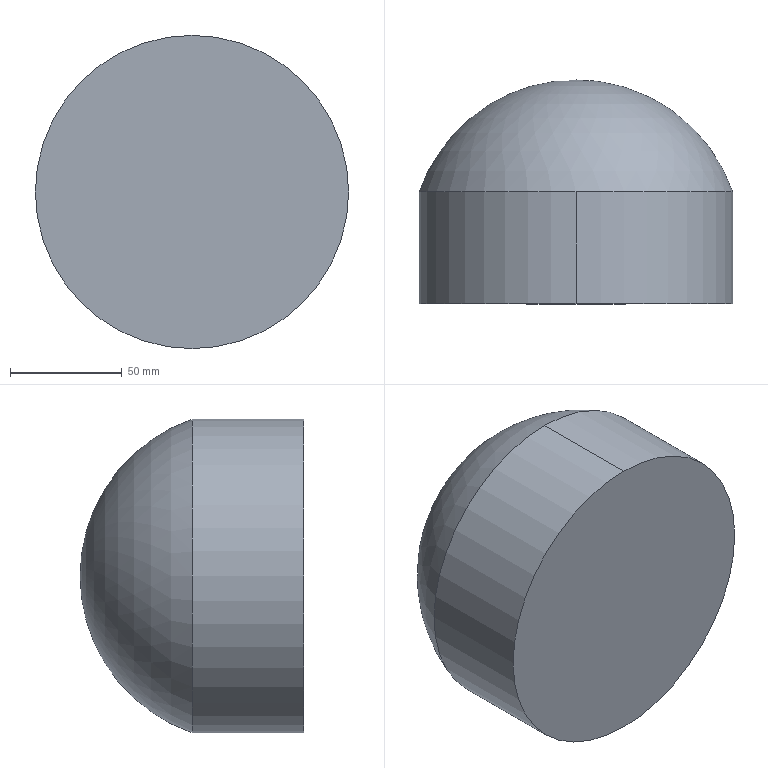Part | SolidWorks | features Dome 1, Extrusion 1 | 1 solid | 4 faces | box 140 x 100 x 140 mm | volume 1219985 mm3 | cylinder 2 | sphere 1 | plane 1 | commonest cylinder face diameters 140 x2
STEP:
#1=CARTESIAN_POINT('',(0.,50.,70.));
#2=VERTEX_POINT('',#1);
#3=CARTESIAN_POINT('',(0.,50.,-70.));
#4=VERTEX_POINT('',#3);
#5=CARTESIAN_POINT('',(0.,50.,0.));
#6=DIRECTION('',(0.,1.,0.));
#7=DIRECTION('',(0.,0.,1.));
#8=AXIS2_PLACEMENT_3D('',#5,#6,#7);
#9=CIRCLE('',#8,70.);
#10=EDGE_CURVE('',#2,#4,#9,.T.);
#11=ORIENTED_EDGE('',*,*,#10,.F.);
#12=CARTESIAN_POINT('',(0.,0.,70.));
#13=VERTEX_POINT('',#12);
#14=CARTESIAN_POINT('',(0.,50.,70.));
#15=DIRECTION('',(0.,-1.,0.));
#16=VECTOR('',#15,1000.);
#17=LINE('',#14,#16);
#18=EDGE_CURVE('',#2,#13,#17,.T.);
#19=ORIENTED_EDGE('',*,*,#18,.T.);
#20=CARTESIAN_POINT('',(0.,0.,-70.));
#21=VERTEX_POINT('',#20);
#22=CARTESIAN_POINT('',(0.,0.,0.));
#23=DIRECTION('',(0.,1.,0.));
#24=DIRECTION('',(0.,0.,1.));
#25=AXIS2_PLACEMENT_3D('',#22,#23,#24);
#26=CIRCLE('',#25,70.);
#27=EDGE_CURVE('',#13,#21,#26,.T.);
#28=ORIENTED_EDGE('',*,*,#27,.T.);
#29=CARTESIAN_POINT('',(0.,50.,-70.));
#30=DIRECTION('',(0.,-1.,0.));
#31=VECTOR('',#30,1000.);
#32=LINE('',#29,#31);
#33=EDGE_CURVE('',#4,#21,#32,.T.);
#34=ORIENTED_EDGE('',*,*,#33,.F.);
#35=EDGE_LOOP('',(#11,#19,#28,#34));
#36=FACE_OUTER_BOUND('',#35,.T.);
#37=CARTESIAN_POINT('',(0.,50.,0.));
#38=DIRECTION('',(0.,-1.,0.));
#39=DIRECTION('',(0.,0.,-1.));
#40=AXIS2_PLACEMENT_3D('',#37,#38,#39);
#41=CYLINDRICAL_SURFACE('',#40,70.);
#42=ADVANCED_FACE('',(#36),#41,.T.);
#43=ORIENTED_EDGE('',*,*,#18,.F.);
#44=CARTESIAN_POINT('',(0.,50.,0.));
#45=DIRECTION('',(0.,1.,0.));
#46=DIRECTION('',(0.,0.,1.));
#47=AXIS2_PLACEMENT_3D('',#44,#45,#46);
#48=CIRCLE('',#47,70.);
#49=EDGE_CURVE('',#4,#2,#48,.T.);
#50=ORIENTED_EDGE('',*,*,#49,.F.);
#51=ORIENTED_EDGE('',*,*,#33,.T.);
#52=CARTESIAN_POINT('',(0.,0.,0.));
#53=DIRECTION('',(0.,1.,0.));
#54=DIRECTION('',(0.,0.,1.));
#55=AXIS2_PLACEMENT_3D('',#52,#53,#54);
#56=CIRCLE('',#55,70.);
#57=EDGE_CURVE('',#21,#13,#56,.T.);
#58=ORIENTED_EDGE('',*,*,#57,.T.);
#59=EDGE_LOOP('',(#43,#50,#51,#58));
#60=FACE_OUTER_BOUND('',#59,.T.);
#61=CARTESIAN_POINT('',(0.,50.,0.));
#62=DIRECTION('',(0.,-1.,0.));
#63=DIRECTION('',(0.,0.,-1.));
#64=AXIS2_PLACEMENT_3D('',#61,#62,#63);
#65=CYLINDRICAL_SURFACE('',#64,70.);
#66=ADVANCED_FACE('',(#60),#65,.T.);
#67=ORIENTED_EDGE('',*,*,#49,.T.);
#68=ORIENTED_EDGE('',*,*,#10,.T.);
#69=EDGE_LOOP('',(#67,#68));
#70=FACE_OUTER_BOUND('',#69,.T.);
#71=CARTESIAN_POINT('',(0.,26.,0.));
#72=DIRECTION('',(0.,1.,0.));
#73=DIRECTION('',(1.,0.,0.));
#74=AXIS2_PLACEMENT_3D('',#71,#72,#73);
#75=SPHERICAL_SURFACE('',#74,74.);
#76=ADVANCED_FACE('',(#70),#75,.T.);
#77=ORIENTED_EDGE('',*,*,#57,.F.);
#78=ORIENTED_EDGE('',*,*,#27,.F.);
#79=EDGE_LOOP('',(#77,#78));
#80=FACE_OUTER_BOUND('',#79,.T.);
#81=CARTESIAN_POINT('',(0.,0.,0.));
#82=DIRECTION('',(0.,1.,0.));
#83=DIRECTION('',(0.,0.,1.));
#84=AXIS2_PLACEMENT_3D('',#81,#82,#83);
#85=PLANE('',#84);
#86=ADVANCED_FACE('',(#80),#85,.F.);
#87=CLOSED_SHELL('',(#42,#66,#76,#86));
#88=MANIFOLD_SOLID_BREP('',#87);
#89=CARTESIAN_POINT('',(0.,0.,0.));
#90=DIRECTION('',(0.,0.,1.));
#91=DIRECTION('',(1.,0.,0.));
#92=AXIS2_PLACEMENT_3D('',#89,#90,#91);
#93=(LENGTH_UNIT()NAMED_UNIT(*)SI_UNIT(.MILLI.,.METRE.));
#94=UNCERTAINTY_MEASURE_WITH_UNIT(LENGTH_MEASURE(0.00001),#93,'','');
#95=(NAMED_UNIT(*)PLANE_ANGLE_UNIT()SI_UNIT($,.RADIAN.));
#96=(NAMED_UNIT(*)SI_UNIT($,.STERADIAN.)SOLID_ANGLE_UNIT());
#97=(GEOMETRIC_REPRESENTATION_CONTEXT(3)GLOBAL_UNCERTAINTY_ASSIGNED_CONTEXT((#94))GLOBAL_UNIT_ASSIGNED_CONTEXT((#93,#95,#96))REPRESENTATION_CONTEXT('',''));
#98=ADVANCED_BREP_SHAPE_REPRESENTATION('',(#88,#92),#97);